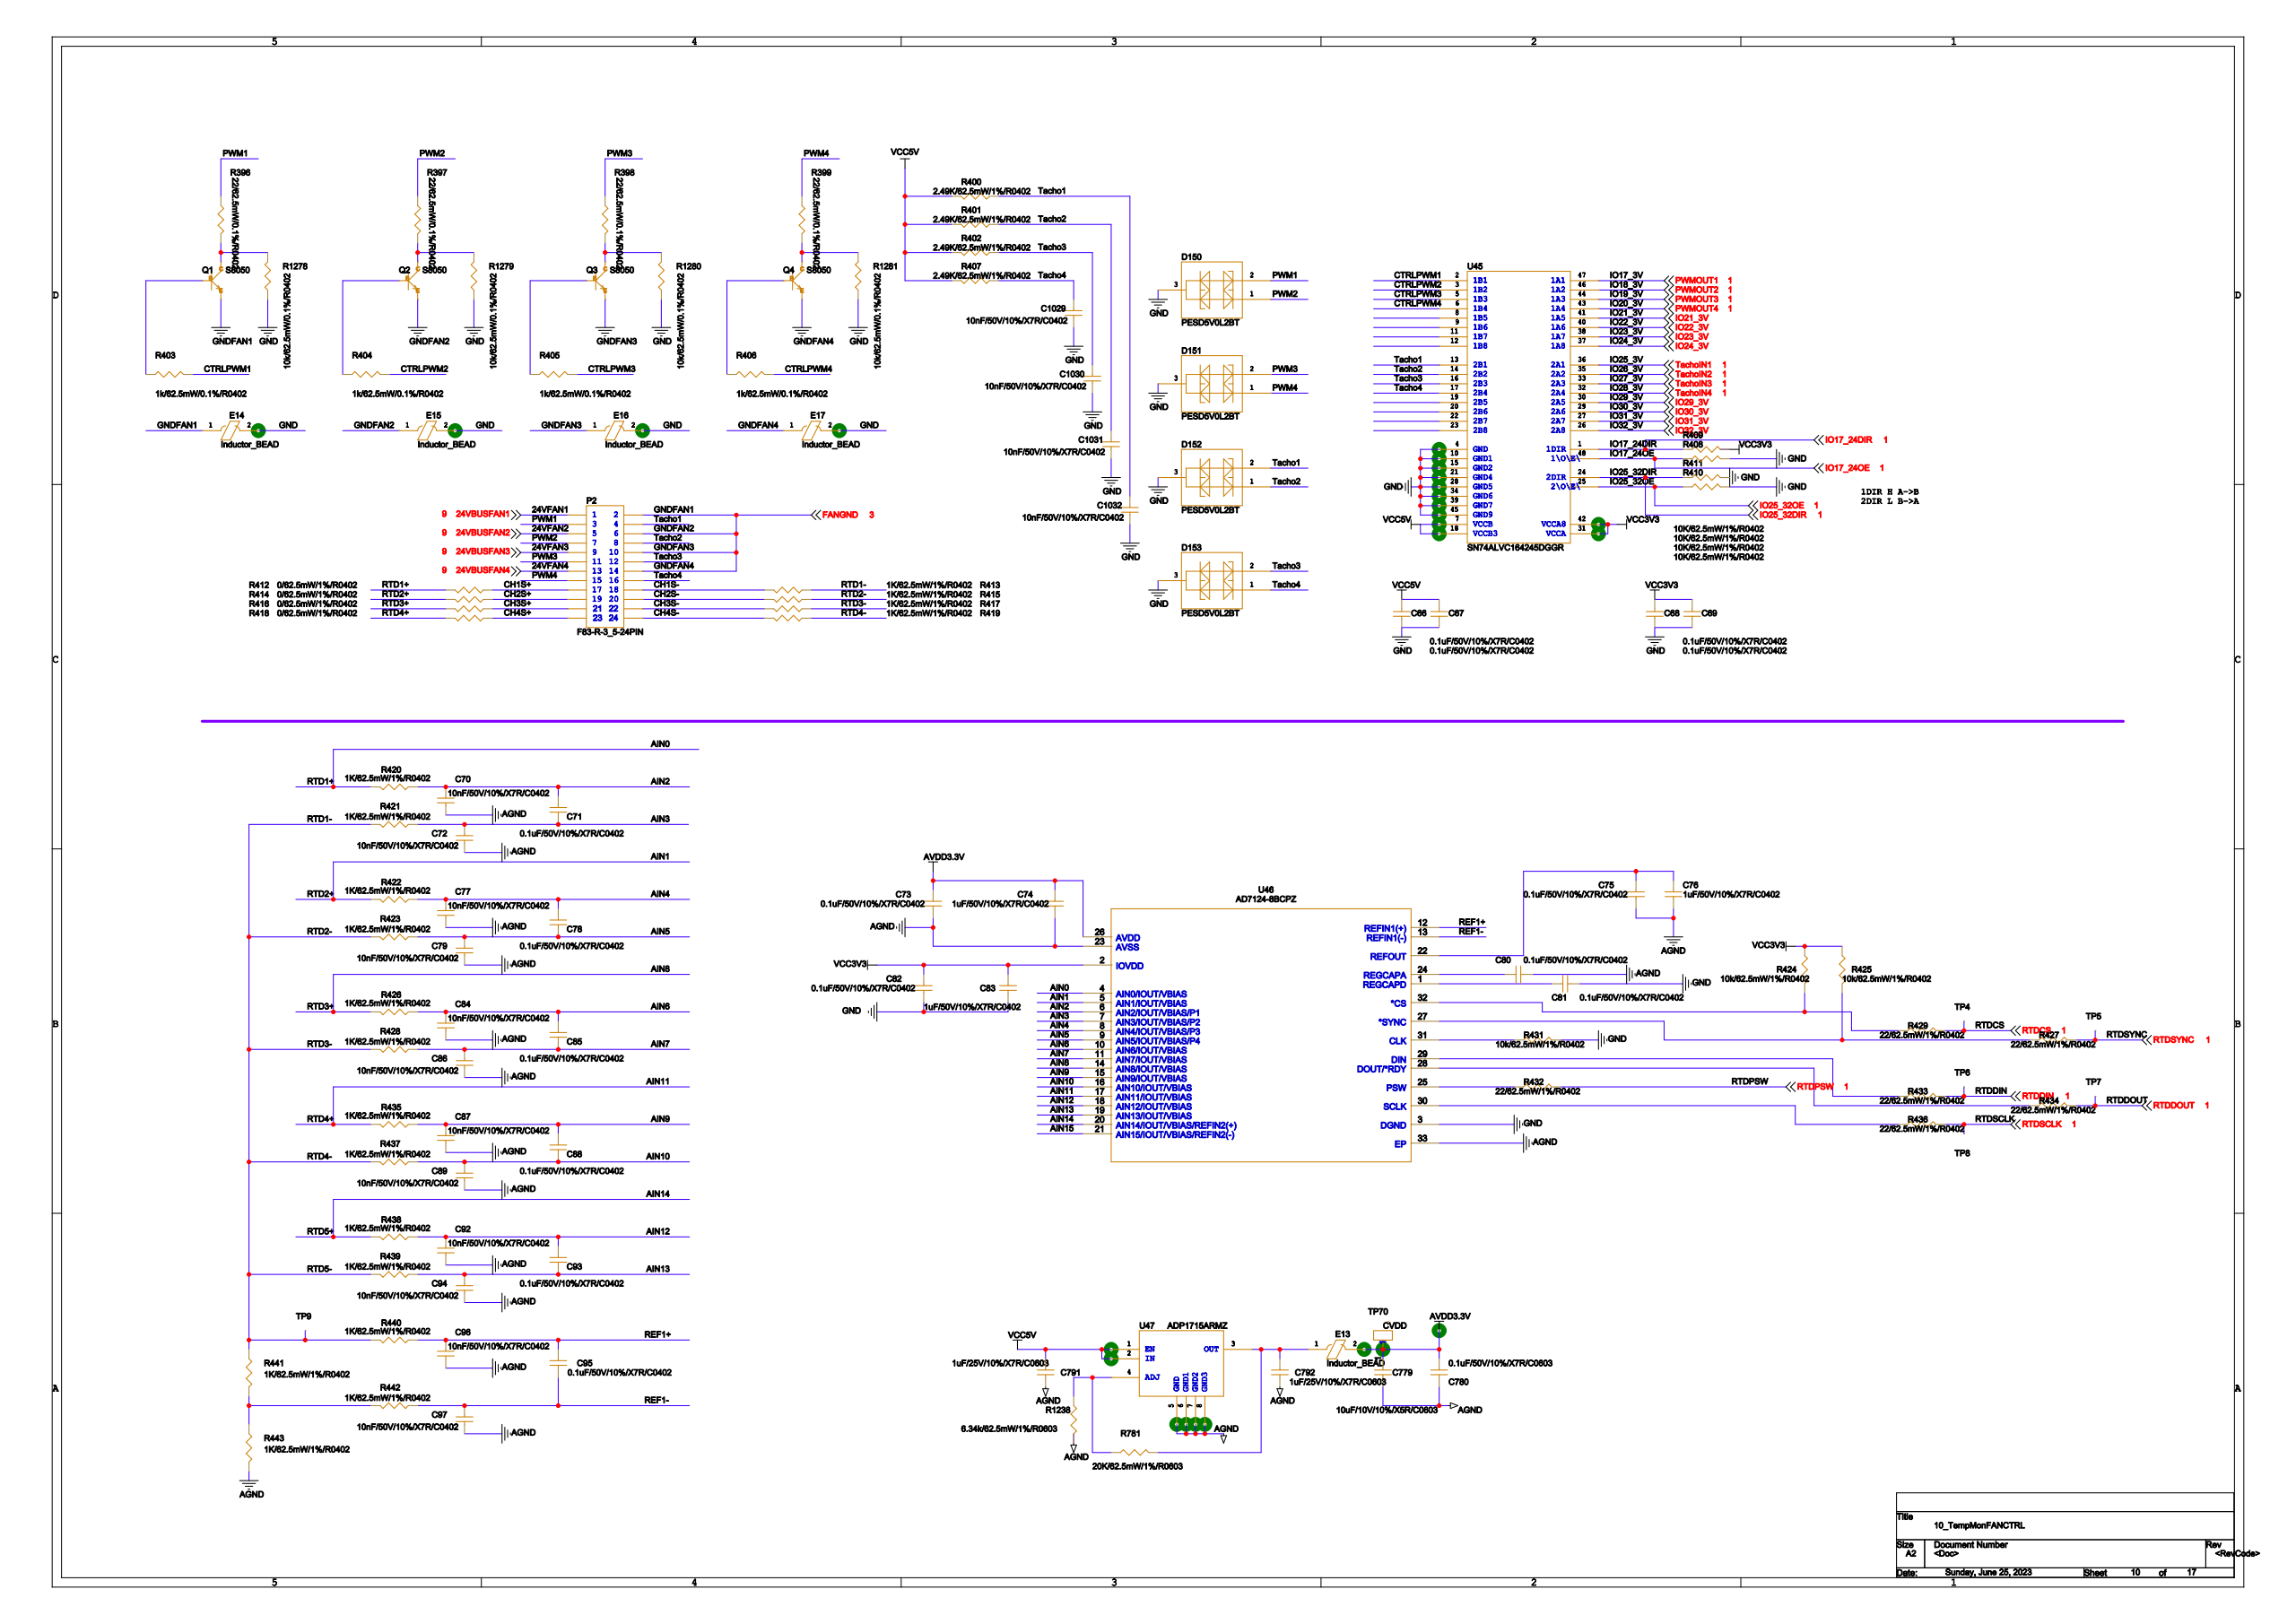Circuit board | Cadence Allegro | 1997 parts | 1536 nets | one sheet of the schematic
Parts on this sheet (reference | value | footprint):
C66 | 0.1uF/50V/10%/X7R/C0402 | 0402
C67 | 0.1uF/50V/10%/X7R/C0402 | 0402
C68 | 0.1uF/50V/10%/X7R/C0402 | 0402
C69 | 0.1uF/50V/10%/X7R/C0402 | 0402
C70 | 10nF/50V/10%/X7R/C0402 | 0402
C71 | 0.1uF/50V/10%/X7R/C0402 | 0402
C72 | 10nF/50V/10%/X7R/C0402 | 0402
C73 | 0.1uF/50V/10%/X7R/C0402 | 0402
C74 | 1uF/50V/10%/X7R/C0402 | 0402
C75 | 0.1uF/50V/10%/X7R/C0402 | 0402
C76 | 1uF/50V/10%/X7R/C0402 | 0402
C77 | 10nF/50V/10%/X7R/C0402 | 0402
C78 | 0.1uF/50V/10%/X7R/C0402 | 0402
C79 | 10nF/50V/10%/X7R/C0402 | 0402
C80 | 0.1uF/50V/10%/X7R/C0402 | 0402
C81 | 0.1uF/50V/10%/X7R/C0402 | 0402
C82 | 0.1uF/50V/10%/X7R/C0402 | 0402
C83 | 1uF/50V/10%/X7R/C0402 | 0402
C84 | 10nF/50V/10%/X7R/C0402 | 0402
C85 | 0.1uF/50V/10%/X7R/C0402 | 0402
C86 | 10nF/50V/10%/X7R/C0402 | 0402
C87 | 10nF/50V/10%/X7R/C0402 | 0402
C88 | 0.1uF/50V/10%/X7R/C0402 | 0402
C89 | 10nF/50V/10%/X7R/C0402 | 0402
C92 | 10nF/50V/10%/X7R/C0402 | 0402
C93 | 0.1uF/50V/10%/X7R/C0402 | 0402
C94 | 10nF/50V/10%/X7R/C0402 | 0402
C95 | 0.1uF/50V/10%/X7R/C0402 | 0402
C96 | 10nF/50V/10%/X7R/C0402 | 0402
C97 | 10nF/50V/10%/X7R/C0402 | 0402
C779 | 10uF/10V/10%/X5R/C0603 | 0603C
C780 | 0.1uF/50V/10%/X7R/C0603 | 0603C
C791 | 1uF/25V/10%/X7R/C0603 | 0603C
C792 | 1uF/25V/10%/X7R/C0603 | 0603C
C1029 | 10nF/50V/10%/X7R/C0402 | 0402
C1030 | 10nF/50V/10%/X7R/C0402 | 0402
C1031 | 10nF/50V/10%/X7R/C0402 | 0402
C1032 | 10nF/50V/10%/X7R/C0402 | 0402
D150 | PESD5V0L2BT | SOT23
D151 | PESD5V0L2BT | SOT23
D152 | PESD5V0L2BT | SOT23
D153 | PESD5V0L2BT | SOT23
E13 | Inductor_BEAD | 0603R
E14 | Inductor_BEAD | 0603R
E15 | Inductor_BEAD | 0603R
E16 | Inductor_BEAD | 0603R
E17 | Inductor_BEAD | 0603R
P2 | F83-R-3_5-24PIN | F83-R-3_5-24PIN
Q1 | S8050 | SOT-23
Q2 | S8050 | SOT-23
Q3 | S8050 | SOT-23
Q4 | S8050 | SOT-23
R396 | 22/62.5mW/0.1%/R0402 | 0402
R397 | 22/62.5mW/0.1%/R0402 | 0402
R398 | 22/62.5mW/0.1%/R0402 | 0402
R399 | 22/62.5mW/0.1%/R0402 | 0402
R400 | 2.49k/62.5mW/1%/R0402 | 0402
R401 | 2.49k/62.5mW/1%/R0402 | 0402
R402 | 2.49k/62.5mW/1%/R0402 | 0402
R403 | 1k/62.5mW/0.1%/R0402 | 0402
R404 | 1k/62.5mW/0.1%/R0402 | 0402
R405 | 1k/62.5mW/0.1%/R0402 | 0402
R406 | 1k/62.5mW/0.1%/R0402 | 0402
R407 | 2.49k/62.5mW/1%/R0402 | 0402
R408 | 10K/62.5mW/1%/R0402 | 0402
R409 | 10K/62.5mW/1%/R0402 | 0402
R410 | 10K/62.5mW/1%/R0402 | 0402
R411 | 10K/62.5mW/1%/R0402 | 0402
R412 | 0/62.5mW/1%/R0402 | 0402
R413 | 1K/62.5mW/1%/R0402 | 0402
R414 | 0/62.5mW/1%/R0402 | 0402
R415 | 1K/62.5mW/1%/R0402 | 0402
R416 | 0/62.5mW/1%/R0402 | 0402
R417 | 1K/62.5mW/1%/R0402 | 0402
R418 | 0/62.5mW/1%/R0402 | 0402
R419 | 1K/62.5mW/1%/R0402 | 0402
R420 | 1K/62.5mW/1%/R0402 | 0402
R421 | 1K/62.5mW/1%/R0402 | 0402
R422 | 1K/62.5mW/1%/R0402 | 0402
R423 | 1K/62.5mW/1%/R0402 | 0402
R424 | 10k/62.5mW/1%/R0402 | 0402
R425 | 10k/62.5mW/1%/R0402 | 0402
R426 | 1K/62.5mW/1%/R0402 | 0402
R427 | 22/62.5mW/1%/R0402 | 0402
R428 | 1K/62.5mW/1%/R0402 | 0402
R429 | 22/62.5mW/1%/R0402 | 0402
R431 | 10k/62.5mW/1%/R0402 | 0402
R432 | 22/62.5mW/1%/R0402 | 0402
R433 | 22/62.5mW/1%/R0402 | 0402
R434 | 22/62.5mW/1%/R0402 | 0402
R435 | 1K/62.5mW/1%/R0402 | 0402
R436 | 22/62.5mW/1%/R0402 | 0402
R437 | 1K/62.5mW/1%/R0402 | 0402
R438 | 1K/62.5mW/1%/R0402 | 0402
R439 | 1K/62.5mW/1%/R0402 | 0402
R440 | 1K/62.5mW/1%/R0402 | 0402
R441 | 1K/62.5mW/1%/R0402 | 0402
R442 | 1K/62.5mW/1%/R0402 | 0402
R443 | 1K/62.5mW/1%/R0402 | 0402
R781 | 20K/62.5mW/1%/R0603 | 0603R
R1238 | 6.34k/62.5mW/1%/R0603 | 0603R
R1278 | 10k/62.5mW/0.1%/R0402 | 0402
R1279 | 10k/62.5mW/0.1%/R0402 | 0402
R1280 | 10k/62.5mW/0.1%/R0402 | 0402
R1281 | 10k/62.5mW/0.1%/R0402 | 0402
TP4 | TEST POINT A | TEST_12MM
TP5 | TEST POINT A | TEST_12MM
TP6 | TEST POINT A | TEST_12MM
TP7 | TEST POINT A | TEST_12MM
TP8 | TEST POINT A | TEST_12MM
TP9 | TEST POINT A | TEST_12MM
TP70 | CVDD | D0_6
U45 | SN74ALVC164245DGGR | TSSOP-48
U46 | Value | CP_32_12_ADI
U47 | ADP1715ARMZ | MSOP8
Nets of these parts (net: part-pin ...):
3.3V: C68-2 C69-2 C82-1 C83-1 R409-1 R424-1 R425-1 U45-31 U45-42 U46-2
AGND: C66-1 C67-1 C68-1 C69-1 C70-2 C72-2 C73-2 C74-2 C75-2 C76-2 C77-2 C79-2 C80-2 C81-2 C82-2 C83-2 C84-2 C86-2 C87-2 C89-2 C92-2 C94-2 C96-2 C97-2 C779-2 C780-2 C791-2 C792-2 C1029-2 C1030-2 C1031-2 C1032-2 D150-3 D151-3 D152-3 D153-3 E14-2 E15-2 E16-2 E17-2 R408-1 R410-1 R411-1 R431-2 R443-2 R1238-1 R1278-1 R1279-1 R1280-1 R1281-1 U47-5 U47-6 U47-7 U47-8 U45-4 U45-10 U45-15 U45-21 U45-28 U45-34 U45-39 U45-45 U46-3 U46-23 U46-33
RTDCS: R429-2 TP4-1
RTDSCLK: R436-2 TP8-1
RTDDIN: R433-2 TP6-1
RTDDOUT: R434-2 TP7-1
RTDSYNC: R427-2 TP5-1
RTDPSW: R432-2
IO25_32DIR: R411-2 U45-24
VCC5V: C66-2 C67-2 C791-1 R400-2 R401-2 R402-2 R407-2 U47-1 U47-2 U45-7 U45-18
IO17_24OE: R408-2 U45-48
PWMOUT1: U45-47
PWMOUT2: U45-46
PWMOUT3: U45-44
PWMOUT4: U45-43
IO25_32OE: R410-2 U45-25
IO17_24DIR: R409-2 U45-1
N24572238: Q1-3 R396-2 R1278-2
N24572234: Q2-3 R397-2 R1279-2
N24572230: Q3-3 R398-2 R1280-2
N24572226: Q4-3 R399-2 R1281-2
N24572323: Q1-1 R403-1
CTRLPWM1: R403-2 U45-2
N24572337: Q2-1 R404-1
CTRLPWM2: R404-2 U45-3
N24572368: Q3-1 R405-1
CTRLPWM3: R405-2 U45-5
N24572399: Q4-1 R406-1
CTRLPWM4: R406-2 U45-6
TACHO1: C1032-1 D152-2 R400-1 P2-4 U45-13
TACHO2: C1031-1 D152-1 R401-1 P2-8 U45-14
TACHO3: C1030-1 D153-2 R402-1 P2-12 U45-16
TACHO4: C1029-1 D153-1 R407-1 P2-16 U45-17
24VBUSFAN1: P2-1
FANGND: E14-1 E15-1 E16-1 E17-1 Q1-2 Q2-2 Q3-2 Q4-2 P2-2 P2-6 P2-10 P2-14
PWM3: D151-2 R398-1 P2-11
24VBUSFAN4: P2-13
PWM4: D151-1 R399-1 P2-15
CH1S+: R412-1 P2-17
CH1S-: R413-2 P2-18
CH2S+: R414-1 P2-19
CH2S-: R415-2 P2-20
CH3S+: R416-1 P2-21
CH3S-: R417-2 P2-22
CH4S+: R418-1 P2-23
CH4S-: R419-2 P2-24
PWM1: D150-2 R396-1 P2-3
24VBUSFAN2: P2-5
PWM2: D150-1 R397-1 P2-7
24VBUSFAN3: P2-9
AVDD3.3V: C73-1 C74-1 C779-1 C780-1 E13-2 TP70-1 U46-26
N23528814: C792-1 E13-1 R781-1 U47-3
N23528786: R781-2 R1238-2 U47-4
AIN2: C70-1 C71-1 R420-1 U46-6
AIN3: C71-2 C72-1 R421-1 U46-7
N23186471: C75-1 C76-1 U46-22
AIN4: C77-1 C78-1 R422-1 U46-8
AIN5: C78-2 C79-1 R423-1 U46-9
N23186180: C80-1 U46-24
N23186182: C81-1 U46-1
AIN6: C84-1 C85-1 R426-1 U46-10
AIN7: C85-2 C86-1 R428-1 U46-11
AIN9: C87-1 C88-1 R435-1 U46-15
AIN10: C88-2 C89-1 R437-1 U46-16
AIN12: C92-1 C93-1 R438-1 U46-18
AIN13: C93-2 C94-1 R439-1 U46-19
REF1+: C95-1 C96-1 R440-1 U46-12
REF1-: C95-2 C97-1 R442-1 U46-13
RTD1-: R413-1 R415-1 R417-1 R419-1 R421-2 R423-2 R428-2 R437-2 R439-2 R440-2 R441-1 TP9-1
AIN0: R412-2 R420-2 U46-4
AIN1: R414-2 R422-2 U46-5
AIN8: R416-2 R426-2 U46-14
AIN11: R418-2 R435-2 U46-17
AIN14: R438-2 U46-20
N23184433: R441-2 R442-2 R443-1
N23186319: R424-2 R429-1 U46-32
N23186325: R425-2 R427-1 U46-27
N23186239: R431-1 U46-31
N23186243: R432-1 U46-25
N23186381: R433-1 U46-29
N23186383: R434-1 U46-28
N23186389: R436-1 U46-30
IO21_3V: U45-41
IO22_3V: U45-40
IO23_3V: U45-38
IO24_3V: U45-37
IO29_3V: U45-30
IO30_3V: U45-29
IO31_3V: U45-27
IO32_3V: U45-26
AIN15: U46-21